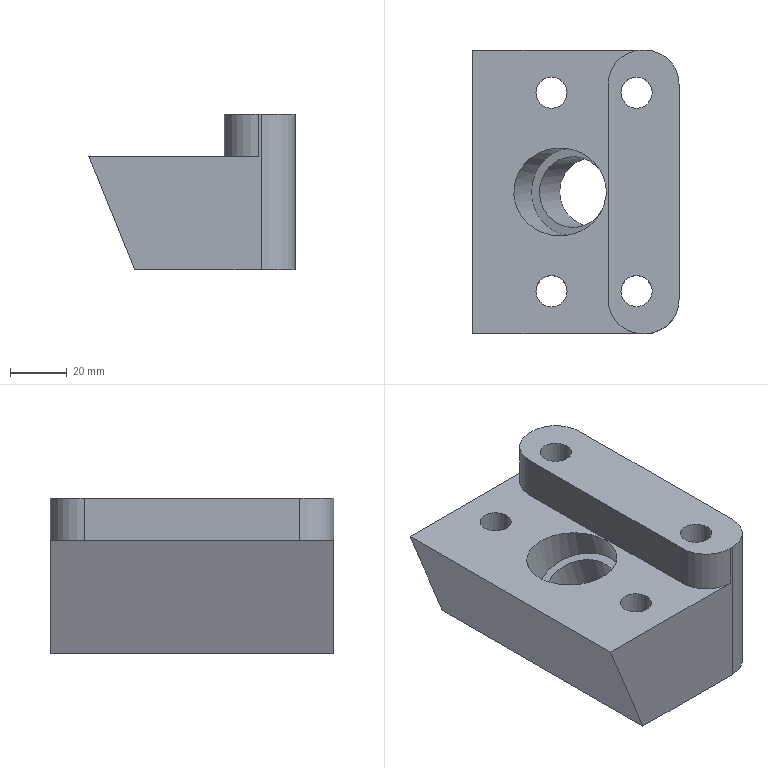Part | STEP file | solid 28 | 1 solid | 27 faces | box 72.72 x 100 x 55.001 mm | volume 242059 mm3 | plane 13 | cylinder 13 | spline 1 | commonest cylinder face diameters 11 x4 18 x4 24 x4 25 x1